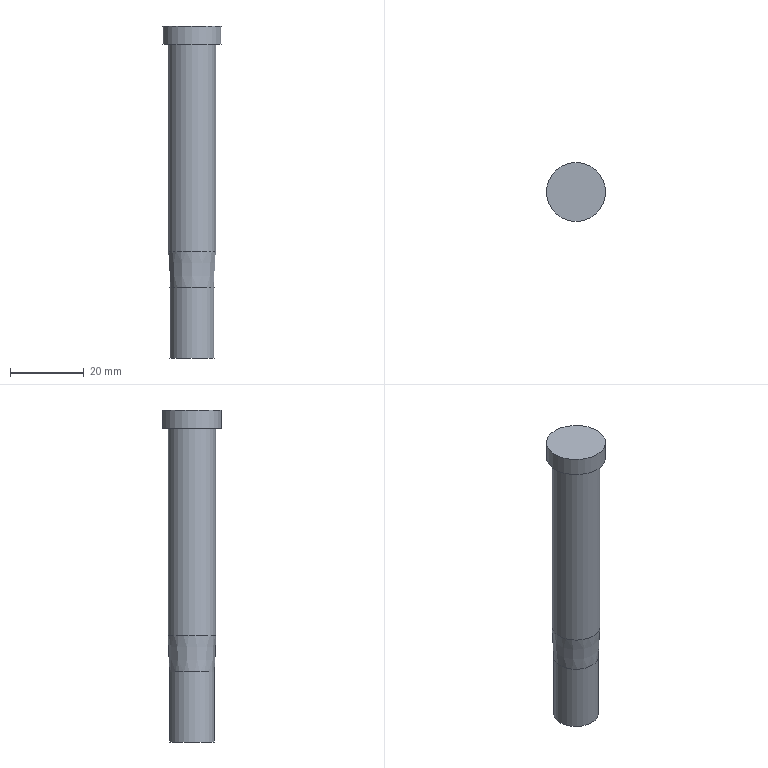Part | NX | features solid 2 | 1 solid | 7 faces | box 16 x 16 x 90 mm | volume 11861 mm3 | plane 3 | cylinder 3 | cone 1 | commonest cylinder face diameters 12.1 x1 13 x1 16 x1
STEP:
#1=CARTESIAN_POINT('',(-319.074,-423.454,92.6));
#2=VERTEX_POINT('',#1);
#3=CARTESIAN_POINT('',(-319.074,-429.504,92.6));
#4=DIRECTION('',(0.,0.,1.));
#5=DIRECTION('',(0.,1.,0.));
#6=AXIS2_PLACEMENT_3D('',#3,#4,#5);
#7=CIRCLE('',#6,6.05);
#8=EDGE_CURVE('',#2,#2,#7,.T.);
#9=ORIENTED_EDGE('',*,*,#8,.F.);
#10=EDGE_LOOP('',(#9));
#11=FACE_BOUND('',#10,.T.);
#12=CARTESIAN_POINT('',(-319.074,-429.504,92.6));
#13=DIRECTION('',(0.,0.,-1.));
#14=DIRECTION('',(0.,-1.,0.));
#15=AXIS2_PLACEMENT_3D('',#12,#13,#14);
#16=PLANE('',#15);
#17=ADVANCED_FACE('',(#11),#16,.T.);
#18=CARTESIAN_POINT('',(-319.074,-423.454,111.6));
#19=VERTEX_POINT('',#18);
#20=CARTESIAN_POINT('',(-319.074,-429.504,111.6));
#21=DIRECTION('',(0.,0.,1.));
#22=DIRECTION('',(0.,1.,0.));
#23=AXIS2_PLACEMENT_3D('',#20,#21,#22);
#24=CIRCLE('',#23,6.05);
#25=EDGE_CURVE('',#19,#19,#24,.T.);
#26=ORIENTED_EDGE('',*,*,#25,.F.);
#27=EDGE_LOOP('',(#26));
#28=FACE_BOUND('',#27,.T.);
#29=ORIENTED_EDGE('',*,*,#8,.T.);
#30=EDGE_LOOP('',(#29));
#31=FACE_BOUND('',#30,.T.);
#32=CARTESIAN_POINT('',(-319.074,-429.504,92.6));
#33=DIRECTION('',(0.,0.,1.));
#34=DIRECTION('',(0.,1.,0.));
#35=AXIS2_PLACEMENT_3D('',#32,#33,#34);
#36=CYLINDRICAL_SURFACE('',#35,6.05);
#37=ADVANCED_FACE('',(#28,#31),#36,.T.);
#38=ORIENTED_EDGE('',*,*,#25,.T.);
#39=EDGE_LOOP('',(#38));
#40=FACE_BOUND('',#39,.T.);
#41=CARTESIAN_POINT('',(-319.074,-423.004,121.6));
#42=VERTEX_POINT('',#41);
#43=CARTESIAN_POINT('',(-319.074,-429.504,121.6));
#44=DIRECTION('',(0.,0.,1.));
#45=DIRECTION('',(0.,1.,0.));
#46=AXIS2_PLACEMENT_3D('',#43,#44,#45);
#47=CIRCLE('',#46,6.5);
#48=EDGE_CURVE('',#42,#42,#47,.T.);
#49=ORIENTED_EDGE('',*,*,#48,.F.);
#50=EDGE_LOOP('',(#49));
#51=FACE_BOUND('',#50,.T.);
#52=CARTESIAN_POINT('',(-319.074,-429.504,111.6));
#53=DIRECTION('',(0.,0.,1.));
#54=DIRECTION('',(0.,1.,0.));
#55=AXIS2_PLACEMENT_3D('',#52,#53,#54);
#56=CONICAL_SURFACE('',#55,6.05,0.04497);
#57=ADVANCED_FACE('',(#40,#51),#56,.T.);
#58=CARTESIAN_POINT('',(-319.074,-436.004,177.6));
#59=VERTEX_POINT('',#58);
#60=CARTESIAN_POINT('',(-319.074,-429.504,177.6));
#61=DIRECTION('',(0.,0.,-1.));
#62=DIRECTION('',(0.,-1.,0.));
#63=AXIS2_PLACEMENT_3D('',#60,#61,#62);
#64=CIRCLE('',#63,6.5);
#65=EDGE_CURVE('',#59,#59,#64,.F.);
#66=ORIENTED_EDGE('',*,*,#65,.F.);
#67=EDGE_LOOP('',(#66));
#68=FACE_BOUND('',#67,.T.);
#69=ORIENTED_EDGE('',*,*,#48,.T.);
#70=EDGE_LOOP('',(#69));
#71=FACE_BOUND('',#70,.T.);
#72=CARTESIAN_POINT('',(-319.074,-429.504,121.6));
#73=DIRECTION('',(0.,0.,1.));
#74=DIRECTION('',(0.,1.,0.));
#75=AXIS2_PLACEMENT_3D('',#72,#73,#74);
#76=CYLINDRICAL_SURFACE('',#75,6.5);
#77=ADVANCED_FACE('',(#68,#71),#76,.T.);
#78=CARTESIAN_POINT('',(-319.074,-421.504,182.6));
#79=VERTEX_POINT('',#78);
#80=CARTESIAN_POINT('',(-319.074,-429.504,182.6));
#81=DIRECTION('',(0.,0.,1.));
#82=DIRECTION('',(0.,1.,0.));
#83=AXIS2_PLACEMENT_3D('',#80,#81,#82);
#84=CIRCLE('',#83,8.);
#85=EDGE_CURVE('',#79,#79,#84,.F.);
#86=ORIENTED_EDGE('',*,*,#85,.F.);
#87=EDGE_LOOP('',(#86));
#88=FACE_BOUND('',#87,.T.);
#89=CARTESIAN_POINT('',(-319.074,-429.504,182.6));
#90=DIRECTION('',(0.,0.,1.));
#91=DIRECTION('',(0.,1.,0.));
#92=AXIS2_PLACEMENT_3D('',#89,#90,#91);
#93=PLANE('',#92);
#94=ADVANCED_FACE('',(#88),#93,.T.);
#95=ORIENTED_EDGE('',*,*,#65,.T.);
#96=EDGE_LOOP('',(#95));
#97=FACE_BOUND('',#96,.T.);
#98=CARTESIAN_POINT('',(-319.074,-437.504,177.6));
#99=VERTEX_POINT('',#98);
#100=CARTESIAN_POINT('',(-319.074,-429.504,177.6));
#101=DIRECTION('',(0.,0.,-1.));
#102=DIRECTION('',(0.,-1.,0.));
#103=AXIS2_PLACEMENT_3D('',#100,#101,#102);
#104=CIRCLE('',#103,8.);
#105=EDGE_CURVE('',#99,#99,#104,.F.);
#106=ORIENTED_EDGE('',*,*,#105,.F.);
#107=EDGE_LOOP('',(#106));
#108=FACE_BOUND('',#107,.T.);
#109=CARTESIAN_POINT('',(-319.074,-429.504,177.6));
#110=DIRECTION('',(0.,0.,-1.));
#111=DIRECTION('',(0.,-1.,0.));
#112=AXIS2_PLACEMENT_3D('',#109,#110,#111);
#113=PLANE('',#112);
#114=ADVANCED_FACE('',(#97,#108),#113,.T.);
#115=ORIENTED_EDGE('',*,*,#85,.T.);
#116=EDGE_LOOP('',(#115));
#117=FACE_BOUND('',#116,.T.);
#118=ORIENTED_EDGE('',*,*,#105,.T.);
#119=EDGE_LOOP('',(#118));
#120=FACE_BOUND('',#119,.T.);
#121=CARTESIAN_POINT('',(-319.074,-429.504,167.6));
#122=DIRECTION('',(0.,0.,1.));
#123=DIRECTION('',(0.,1.,0.));
#124=AXIS2_PLACEMENT_3D('',#121,#122,#123);
#125=CYLINDRICAL_SURFACE('',#124,8.);
#126=ADVANCED_FACE('',(#117,#120),#125,.T.);
#127=CLOSED_SHELL('',(#17,#37,#57,#77,#94,#114,#126));
#128=MANIFOLD_SOLID_BREP('',#127);
#129=(LENGTH_UNIT()NAMED_UNIT(*)SI_UNIT(.MILLI.,.METRE.));
#130=UNCERTAINTY_MEASURE_WITH_UNIT(LENGTH_MEASURE(0.00001),#129,'','');
#131=(NAMED_UNIT(*)PLANE_ANGLE_UNIT()SI_UNIT($,.RADIAN.));
#132=(NAMED_UNIT(*)SI_UNIT($,.STERADIAN.)SOLID_ANGLE_UNIT());
#133=(GEOMETRIC_REPRESENTATION_CONTEXT(3)GLOBAL_UNCERTAINTY_ASSIGNED_CONTEXT((#130))GLOBAL_UNIT_ASSIGNED_CONTEXT((#129,#131,#132))REPRESENTATION_CONTEXT('',''));
#134=ADVANCED_BREP_SHAPE_REPRESENTATION('',(#128),#133);